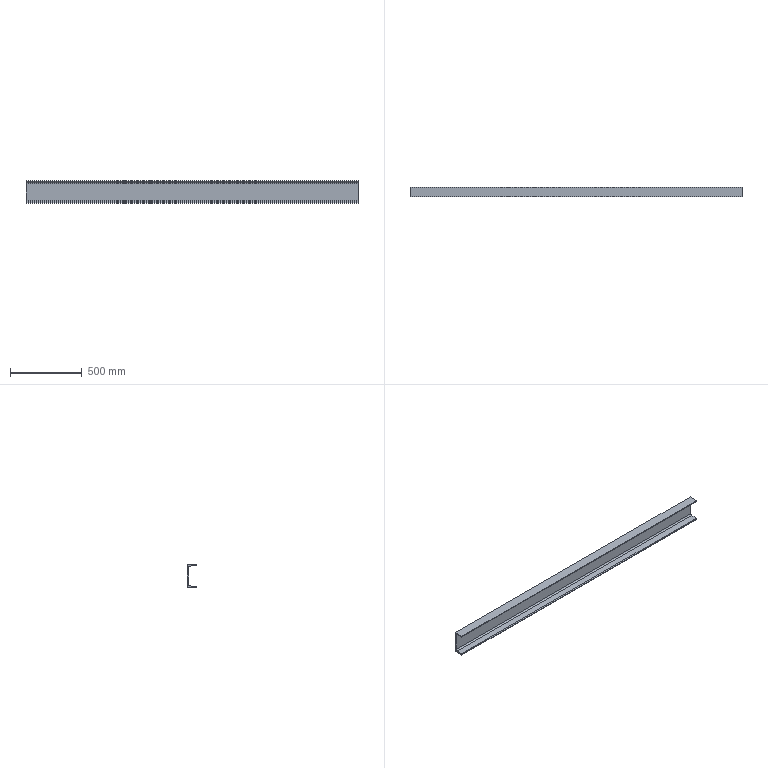Part | STEP file | 08-Channel 100x48_default<machining> | 1 solid | 14 faces | box 2320 x 65 x 160 mm | volume 5777947 mm3 | plane 10 | cylinder 4 | commonest cylinder face diameters 10 x2 20 x2
STEP:
#1=CARTESIAN_POINT('',(0.,0.,0.));
#2=DIRECTION('',(0.,0.,1.));
#3=DIRECTION('',(1.,0.,0.));
#4=AXIS2_PLACEMENT_3D('',#1,#2,#3);
#5=CARTESIAN_POINT('',(0.,-65.,-160.));
#6=VERTEX_POINT('',#5);
#7=CARTESIAN_POINT('',(0.,0.,-160.));
#8=VERTEX_POINT('',#7);
#9=CARTESIAN_POINT('',(0.,0.,-160.));
#10=DIRECTION('',(0.,1.,0.));
#11=VECTOR('',#10,1.);
#12=LINE('',#9,#11);
#13=CARTESIAN_POINT('',(2320.,0.,-160.));
#14=DIRECTION('',(0.,0.,1.));
#15=DIRECTION('',(1.,0.,0.));
#16=AXIS2_PLACEMENT_3D('',#13,#14,#15);
#17=PLANE('',#16);
#18=CARTESIAN_POINT('',(-2320.,0.));
#19=DIRECTION('',(0.,1.));
#20=VECTOR('',#19,1.);
#21=LINE('',#18,#20);
#22=(GEOMETRIC_REPRESENTATION_CONTEXT(2)PARAMETRIC_REPRESENTATION_CONTEXT()REPRESENTATION_CONTEXT('',''));
#23=DEFINITIONAL_REPRESENTATION('',(#21),#22);
#24=PCURVE('',#17,#23);
#25=CARTESIAN_POINT('',(0.,-60.,-156.59));
#26=DIRECTION('',(1.,0.,0.));
#27=DIRECTION('',(0.,0.,-1.));
#28=AXIS2_PLACEMENT_3D('',#25,#26,#27);
#29=PLANE('',#28);
#30=CARTESIAN_POINT('',(3.41,60.));
#31=DIRECTION('',(0.,1.));
#32=VECTOR('',#31,1.);
#33=LINE('',#30,#32);
#34=(GEOMETRIC_REPRESENTATION_CONTEXT(2)PARAMETRIC_REPRESENTATION_CONTEXT()REPRESENTATION_CONTEXT('',''));
#35=DEFINITIONAL_REPRESENTATION('',(#33),#34);
#36=PCURVE('',#29,#35);
#37=SURFACE_CURVE('',#12,(#24,#36),.PCURVE_S1.);
#38=EDGE_CURVE('',#6,#8,#37,.T.);
#39=ORIENTED_EDGE('',*,*,#38,.T.);
#40=CARTESIAN_POINT('',(2320.,0.,-160.));
#41=VERTEX_POINT('',#40);
#42=CARTESIAN_POINT('',(2320.,0.,-160.));
#43=DIRECTION('',(-1.,0.,0.));
#44=VECTOR('',#43,1.);
#45=LINE('',#42,#44);
#46=CARTESIAN_POINT('',(0.,0.));
#47=DIRECTION('',(-1.,0.));
#48=VECTOR('',#47,1.);
#49=LINE('',#46,#48);
#50=(GEOMETRIC_REPRESENTATION_CONTEXT(2)PARAMETRIC_REPRESENTATION_CONTEXT()REPRESENTATION_CONTEXT('',''));
#51=DEFINITIONAL_REPRESENTATION('',(#49),#50);
#52=PCURVE('',#17,#51);
#53=CARTESIAN_POINT('',(2320.,0.,0.));
#54=DIRECTION('',(0.,-1.,0.));
#55=DIRECTION('',(0.,0.,-1.));
#56=AXIS2_PLACEMENT_3D('',#53,#54,#55);
#57=PLANE('',#56);
#58=CARTESIAN_POINT('',(160.,0.));
#59=DIRECTION('',(0.,-1.));
#60=VECTOR('',#59,1.);
#61=LINE('',#58,#60);
#62=(GEOMETRIC_REPRESENTATION_CONTEXT(2)PARAMETRIC_REPRESENTATION_CONTEXT()REPRESENTATION_CONTEXT('',''));
#63=DEFINITIONAL_REPRESENTATION('',(#61),#62);
#64=PCURVE('',#57,#63);
#65=SURFACE_CURVE('',#45,(#52,#64),.PCURVE_S1.);
#66=EDGE_CURVE('',#41,#8,#65,.T.);
#67=ORIENTED_EDGE('',*,*,#66,.F.);
#68=CARTESIAN_POINT('',(2320.,-65.,-160.));
#69=VERTEX_POINT('',#68);
#70=CARTESIAN_POINT('',(2320.,0.,-160.));
#71=DIRECTION('',(0.,1.,0.));
#72=VECTOR('',#71,1.);
#73=LINE('',#70,#72);
#74=CARTESIAN_POINT('',(0.,0.));
#75=DIRECTION('',(0.,1.));
#76=VECTOR('',#75,1.);
#77=LINE('',#74,#76);
#78=(GEOMETRIC_REPRESENTATION_CONTEXT(2)PARAMETRIC_REPRESENTATION_CONTEXT()REPRESENTATION_CONTEXT('',''));
#79=DEFINITIONAL_REPRESENTATION('',(#77),#78);
#80=PCURVE('',#17,#79);
#81=CARTESIAN_POINT('',(2320.,-60.,-156.59));
#82=DIRECTION('',(1.,0.,0.));
#83=DIRECTION('',(0.,0.,-1.));
#84=AXIS2_PLACEMENT_3D('',#81,#82,#83);
#85=PLANE('',#84);
#86=CARTESIAN_POINT('',(3.41,60.));
#87=DIRECTION('',(0.,1.));
#88=VECTOR('',#87,1.);
#89=LINE('',#86,#88);
#90=(GEOMETRIC_REPRESENTATION_CONTEXT(2)PARAMETRIC_REPRESENTATION_CONTEXT()REPRESENTATION_CONTEXT('',''));
#91=DEFINITIONAL_REPRESENTATION('',(#89),#90);
#92=PCURVE('',#85,#91);
#93=SURFACE_CURVE('',#73,(#80,#92),.PCURVE_S1.);
#94=EDGE_CURVE('',#69,#41,#93,.T.);
#95=ORIENTED_EDGE('',*,*,#94,.F.);
#96=CARTESIAN_POINT('',(2320.,-65.,-160.));
#97=DIRECTION('',(-1.,0.,0.));
#98=VECTOR('',#97,1.);
#99=LINE('',#96,#98);
#100=CARTESIAN_POINT('',(0.,-65.));
#101=DIRECTION('',(-1.,0.));
#102=VECTOR('',#101,1.);
#103=LINE('',#100,#102);
#104=(GEOMETRIC_REPRESENTATION_CONTEXT(2)PARAMETRIC_REPRESENTATION_CONTEXT()REPRESENTATION_CONTEXT('',''));
#105=DEFINITIONAL_REPRESENTATION('',(#103),#104);
#106=PCURVE('',#17,#105);
#107=CARTESIAN_POINT('',(2320.,-65.,-156.59));
#108=DIRECTION('',(0.,1.,0.));
#109=DIRECTION('',(0.,0.,1.));
#110=AXIS2_PLACEMENT_3D('',#107,#108,#109);
#111=PLANE('',#110);
#112=CARTESIAN_POINT('',(-3.41,0.));
#113=DIRECTION('',(0.,-1.));
#114=VECTOR('',#113,1.);
#115=LINE('',#112,#114);
#116=(GEOMETRIC_REPRESENTATION_CONTEXT(2)PARAMETRIC_REPRESENTATION_CONTEXT()REPRESENTATION_CONTEXT('',''));
#117=DEFINITIONAL_REPRESENTATION('',(#115),#116);
#118=PCURVE('',#111,#117);
#119=SURFACE_CURVE('',#99,(#106,#118),.PCURVE_S1.);
#120=EDGE_CURVE('',#69,#6,#119,.T.);
#121=ORIENTED_EDGE('',*,*,#120,.T.);
#122=EDGE_LOOP('',(#39,#67,#95,#121));
#123=FACE_BOUND('',#122,.T.);
#124=ADVANCED_FACE('',(#123),#17,.F.);
#125=CARTESIAN_POINT('',(0.,0.,0.));
#126=VERTEX_POINT('',#125);
#127=CARTESIAN_POINT('',(0.,0.,0.));
#128=DIRECTION('',(0.,0.,1.));
#129=VECTOR('',#128,1.);
#130=LINE('',#127,#129);
#131=CARTESIAN_POINT('',(0.,-2320.));
#132=DIRECTION('',(-1.,0.));
#133=VECTOR('',#132,1.);
#134=LINE('',#131,#133);
#135=(GEOMETRIC_REPRESENTATION_CONTEXT(2)PARAMETRIC_REPRESENTATION_CONTEXT()REPRESENTATION_CONTEXT('',''));
#136=DEFINITIONAL_REPRESENTATION('',(#134),#135);
#137=PCURVE('',#57,#136);
#138=CARTESIAN_POINT('',(-156.59,60.));
#139=DIRECTION('',(-1.,0.));
#140=VECTOR('',#139,1.);
#141=LINE('',#138,#140);
#142=(GEOMETRIC_REPRESENTATION_CONTEXT(2)PARAMETRIC_REPRESENTATION_CONTEXT()REPRESENTATION_CONTEXT('',''));
#143=DEFINITIONAL_REPRESENTATION('',(#141),#142);
#144=PCURVE('',#29,#143);
#145=SURFACE_CURVE('',#130,(#137,#144),.PCURVE_S1.);
#146=EDGE_CURVE('',#8,#126,#145,.T.);
#147=ORIENTED_EDGE('',*,*,#146,.T.);
#148=CARTESIAN_POINT('',(2320.,0.,0.));
#149=VERTEX_POINT('',#148);
#150=CARTESIAN_POINT('',(2320.,0.,0.));
#151=DIRECTION('',(-1.,0.,0.));
#152=VECTOR('',#151,1.);
#153=LINE('',#150,#152);
#154=CARTESIAN_POINT('',(0.,0.));
#155=DIRECTION('',(0.,-1.));
#156=VECTOR('',#155,1.);
#157=LINE('',#154,#156);
#158=(GEOMETRIC_REPRESENTATION_CONTEXT(2)PARAMETRIC_REPRESENTATION_CONTEXT()REPRESENTATION_CONTEXT('',''));
#159=DEFINITIONAL_REPRESENTATION('',(#157),#158);
#160=PCURVE('',#57,#159);
#161=CARTESIAN_POINT('',(2320.,0.,0.));
#162=DIRECTION('',(0.,0.,-1.));
#163=DIRECTION('',(0.,1.,0.));
#164=AXIS2_PLACEMENT_3D('',#161,#162,#163);
#165=PLANE('',#164);
#166=CARTESIAN_POINT('',(0.,0.));
#167=DIRECTION('',(0.,-1.));
#168=VECTOR('',#167,1.);
#169=LINE('',#166,#168);
#170=(GEOMETRIC_REPRESENTATION_CONTEXT(2)PARAMETRIC_REPRESENTATION_CONTEXT()REPRESENTATION_CONTEXT('',''));
#171=DEFINITIONAL_REPRESENTATION('',(#169),#170);
#172=PCURVE('',#165,#171);
#173=SURFACE_CURVE('',#153,(#160,#172),.PCURVE_S1.);
#174=EDGE_CURVE('',#149,#126,#173,.T.);
#175=ORIENTED_EDGE('',*,*,#174,.F.);
#176=CARTESIAN_POINT('',(2320.,0.,0.));
#177=DIRECTION('',(0.,0.,1.));
#178=VECTOR('',#177,1.);
#179=LINE('',#176,#178);
#180=CARTESIAN_POINT('',(0.,0.));
#181=DIRECTION('',(-1.,0.));
#182=VECTOR('',#181,1.);
#183=LINE('',#180,#182);
#184=(GEOMETRIC_REPRESENTATION_CONTEXT(2)PARAMETRIC_REPRESENTATION_CONTEXT()REPRESENTATION_CONTEXT('',''));
#185=DEFINITIONAL_REPRESENTATION('',(#183),#184);
#186=PCURVE('',#57,#185);
#187=CARTESIAN_POINT('',(-156.59,60.));
#188=DIRECTION('',(-1.,0.));
#189=VECTOR('',#188,1.);
#190=LINE('',#187,#189);
#191=(GEOMETRIC_REPRESENTATION_CONTEXT(2)PARAMETRIC_REPRESENTATION_CONTEXT()REPRESENTATION_CONTEXT('',''));
#192=DEFINITIONAL_REPRESENTATION('',(#190),#191);
#193=PCURVE('',#85,#192);
#194=SURFACE_CURVE('',#179,(#186,#193),.PCURVE_S1.);
#195=EDGE_CURVE('',#41,#149,#194,.T.);
#196=ORIENTED_EDGE('',*,*,#195,.F.);
#197=ORIENTED_EDGE('',*,*,#66,.T.);
#198=EDGE_LOOP('',(#147,#175,#196,#197));
#199=FACE_BOUND('',#198,.T.);
#200=ADVANCED_FACE('',(#199),#57,.F.);
#201=CARTESIAN_POINT('',(0.,-65.,0.));
#202=VERTEX_POINT('',#201);
#203=CARTESIAN_POINT('',(0.,0.,0.));
#204=DIRECTION('',(0.,-1.,0.));
#205=VECTOR('',#204,1.);
#206=LINE('',#203,#205);
#207=CARTESIAN_POINT('',(0.,-2320.));
#208=DIRECTION('',(-1.,0.));
#209=VECTOR('',#208,1.);
#210=LINE('',#207,#209);
#211=(GEOMETRIC_REPRESENTATION_CONTEXT(2)PARAMETRIC_REPRESENTATION_CONTEXT()REPRESENTATION_CONTEXT('',''));
#212=DEFINITIONAL_REPRESENTATION('',(#210),#211);
#213=PCURVE('',#165,#212);
#214=CARTESIAN_POINT('',(-156.59,60.));
#215=DIRECTION('',(0.,-1.));
#216=VECTOR('',#215,1.);
#217=LINE('',#214,#216);
#218=(GEOMETRIC_REPRESENTATION_CONTEXT(2)PARAMETRIC_REPRESENTATION_CONTEXT()REPRESENTATION_CONTEXT('',''));
#219=DEFINITIONAL_REPRESENTATION('',(#217),#218);
#220=PCURVE('',#29,#219);
#221=SURFACE_CURVE('',#206,(#213,#220),.PCURVE_S1.);
#222=EDGE_CURVE('',#126,#202,#221,.T.);
#223=ORIENTED_EDGE('',*,*,#222,.T.);
#224=CARTESIAN_POINT('',(2320.,-65.,0.));
#225=VERTEX_POINT('',#224);
#226=CARTESIAN_POINT('',(2320.,-65.,0.));
#227=DIRECTION('',(-1.,0.,0.));
#228=VECTOR('',#227,1.);
#229=LINE('',#226,#228);
#230=CARTESIAN_POINT('',(-65.,0.));
#231=DIRECTION('',(0.,-1.));
#232=VECTOR('',#231,1.);
#233=LINE('',#230,#232);
#234=(GEOMETRIC_REPRESENTATION_CONTEXT(2)PARAMETRIC_REPRESENTATION_CONTEXT()REPRESENTATION_CONTEXT('',''));
#235=DEFINITIONAL_REPRESENTATION('',(#233),#234);
#236=PCURVE('',#165,#235);
#237=CARTESIAN_POINT('',(2320.,-65.,-3.41));
#238=DIRECTION('',(0.,1.,0.));
#239=DIRECTION('',(0.,0.,1.));
#240=AXIS2_PLACEMENT_3D('',#237,#238,#239);
#241=PLANE('',#240);
#242=CARTESIAN_POINT('',(3.41,0.));
#243=DIRECTION('',(0.,-1.));
#244=VECTOR('',#243,1.);
#245=LINE('',#242,#244);
#246=(GEOMETRIC_REPRESENTATION_CONTEXT(2)PARAMETRIC_REPRESENTATION_CONTEXT()REPRESENTATION_CONTEXT('',''));
#247=DEFINITIONAL_REPRESENTATION('',(#245),#246);
#248=PCURVE('',#241,#247);
#249=SURFACE_CURVE('',#229,(#236,#248),.PCURVE_S1.);
#250=EDGE_CURVE('',#225,#202,#249,.T.);
#251=ORIENTED_EDGE('',*,*,#250,.F.);
#252=CARTESIAN_POINT('',(2320.,0.,0.));
#253=DIRECTION('',(0.,-1.,0.));
#254=VECTOR('',#253,1.);
#255=LINE('',#252,#254);
#256=CARTESIAN_POINT('',(0.,0.));
#257=DIRECTION('',(-1.,0.));
#258=VECTOR('',#257,1.);
#259=LINE('',#256,#258);
#260=(GEOMETRIC_REPRESENTATION_CONTEXT(2)PARAMETRIC_REPRESENTATION_CONTEXT()REPRESENTATION_CONTEXT('',''));
#261=DEFINITIONAL_REPRESENTATION('',(#259),#260);
#262=PCURVE('',#165,#261);
#263=CARTESIAN_POINT('',(-156.59,60.));
#264=DIRECTION('',(0.,-1.));
#265=VECTOR('',#264,1.);
#266=LINE('',#263,#265);
#267=(GEOMETRIC_REPRESENTATION_CONTEXT(2)PARAMETRIC_REPRESENTATION_CONTEXT()REPRESENTATION_CONTEXT('',''));
#268=DEFINITIONAL_REPRESENTATION('',(#266),#267);
#269=PCURVE('',#85,#268);
#270=SURFACE_CURVE('',#255,(#262,#269),.PCURVE_S1.);
#271=EDGE_CURVE('',#149,#225,#270,.T.);
#272=ORIENTED_EDGE('',*,*,#271,.F.);
#273=ORIENTED_EDGE('',*,*,#174,.T.);
#274=EDGE_LOOP('',(#223,#251,#272,#273));
#275=FACE_BOUND('',#274,.T.);
#276=ADVANCED_FACE('',(#275),#165,.F.);
#277=CARTESIAN_POINT('',(0.,-65.,-3.41));
#278=VERTEX_POINT('',#277);
#279=CARTESIAN_POINT('',(0.,-65.,-3.41));
#280=DIRECTION('',(0.,0.,-1.));
#281=VECTOR('',#280,1.);
#282=LINE('',#279,#281);
#283=CARTESIAN_POINT('',(0.,-2320.));
#284=DIRECTION('',(-1.,0.));
#285=VECTOR('',#284,1.);
#286=LINE('',#283,#285);
#287=(GEOMETRIC_REPRESENTATION_CONTEXT(2)PARAMETRIC_REPRESENTATION_CONTEXT()REPRESENTATION_CONTEXT('',''));
#288=DEFINITIONAL_REPRESENTATION('',(#286),#287);
#289=PCURVE('',#241,#288);
#290=CARTESIAN_POINT('',(-153.18,-5.));
#291=DIRECTION('',(1.,0.));
#292=VECTOR('',#291,1.);
#293=LINE('',#290,#292);
#294=(GEOMETRIC_REPRESENTATION_CONTEXT(2)PARAMETRIC_REPRESENTATION_CONTEXT()REPRESENTATION_CONTEXT('',''));
#295=DEFINITIONAL_REPRESENTATION('',(#293),#294);
#296=PCURVE('',#29,#295);
#297=SURFACE_CURVE('',#282,(#289,#296),.PCURVE_S1.);
#298=EDGE_CURVE('',#202,#278,#297,.T.);
#299=ORIENTED_EDGE('',*,*,#298,.T.);
#300=CARTESIAN_POINT('',(2320.,-65.,-3.41));
#301=VERTEX_POINT('',#300);
#302=CARTESIAN_POINT('',(2320.,-65.,-3.41));
#303=DIRECTION('',(-1.,0.,0.));
#304=VECTOR('',#303,1.);
#305=LINE('',#302,#304);
#306=CARTESIAN_POINT('',(0.,0.));
#307=DIRECTION('',(0.,-1.));
#308=VECTOR('',#307,1.);
#309=LINE('',#306,#308);
#310=(GEOMETRIC_REPRESENTATION_CONTEXT(2)PARAMETRIC_REPRESENTATION_CONTEXT()REPRESENTATION_CONTEXT('',''));
#311=DEFINITIONAL_REPRESENTATION('',(#309),#310);
#312=PCURVE('',#241,#311);
#313=CARTESIAN_POINT('',(2320.,-60.,-3.41));
#314=DIRECTION('',(-1.,0.,0.));
#315=DIRECTION('',(0.,0.,1.));
#316=AXIS2_PLACEMENT_3D('',#313,#314,#315);
#317=CYLINDRICAL_SURFACE('',#316,5.);
#318=CARTESIAN_POINT('',(4.712,0.));
#319=DIRECTION('',(0.,1.));
#320=VECTOR('',#319,1.);
#321=LINE('',#318,#320);
#322=(GEOMETRIC_REPRESENTATION_CONTEXT(2)PARAMETRIC_REPRESENTATION_CONTEXT()REPRESENTATION_CONTEXT('',''));
#323=DEFINITIONAL_REPRESENTATION('',(#321),#322);
#324=PCURVE('',#317,#323);
#325=SURFACE_CURVE('',#305,(#312,#324),.PCURVE_S1.);
#326=EDGE_CURVE('',#301,#278,#325,.T.);
#327=ORIENTED_EDGE('',*,*,#326,.F.);
#328=CARTESIAN_POINT('',(2320.,-65.,-3.41));
#329=DIRECTION('',(0.,0.,-1.));
#330=VECTOR('',#329,1.);
#331=LINE('',#328,#330);
#332=CARTESIAN_POINT('',(0.,0.));
#333=DIRECTION('',(-1.,0.));
#334=VECTOR('',#333,1.);
#335=LINE('',#332,#334);
#336=(GEOMETRIC_REPRESENTATION_CONTEXT(2)PARAMETRIC_REPRESENTATION_CONTEXT()REPRESENTATION_CONTEXT('',''));
#337=DEFINITIONAL_REPRESENTATION('',(#335),#336);
#338=PCURVE('',#241,#337);
#339=CARTESIAN_POINT('',(-153.18,-5.));
#340=DIRECTION('',(1.,0.));
#341=VECTOR('',#340,1.);
#342=LINE('',#339,#341);
#343=(GEOMETRIC_REPRESENTATION_CONTEXT(2)PARAMETRIC_REPRESENTATION_CONTEXT()REPRESENTATION_CONTEXT('',''));
#344=DEFINITIONAL_REPRESENTATION('',(#342),#343);
#345=PCURVE('',#85,#344);
#346=SURFACE_CURVE('',#331,(#338,#345),.PCURVE_S1.);
#347=EDGE_CURVE('',#225,#301,#346,.T.);
#348=ORIENTED_EDGE('',*,*,#347,.F.);
#349=ORIENTED_EDGE('',*,*,#250,.T.);
#350=EDGE_LOOP('',(#299,#327,#348,#349));
#351=FACE_BOUND('',#350,.T.);
#352=ADVANCED_FACE('',(#351),#241,.F.);
#353=CARTESIAN_POINT('',(0.,-60.287,-8.402));
#354=VERTEX_POINT('',#353);
#355=CARTESIAN_POINT('',(0.,-60.,-3.41));
#356=DIRECTION('',(1.,0.,0.));
#357=DIRECTION('',(0.,0.,-1.));
#358=AXIS2_PLACEMENT_3D('',#355,#356,#357);
#359=CIRCLE('',#358,5.);
#360=CARTESIAN_POINT('',(9.425,2320.));
#361=DIRECTION('',(-1.,0.));
#362=VECTOR('',#361,1.);
#363=LINE('',#360,#362);
#364=(GEOMETRIC_REPRESENTATION_CONTEXT(2)PARAMETRIC_REPRESENTATION_CONTEXT()REPRESENTATION_CONTEXT('',''));
#365=DEFINITIONAL_REPRESENTATION('',(#363),#364);
#366=PCURVE('',#317,#365);
#367=CARTESIAN_POINT('',(-153.18,0.));
#368=DIRECTION('',(1.,0.));
#369=AXIS2_PLACEMENT_2D('',#367,#368);
#370=CIRCLE('',#369,5.);
#371=(GEOMETRIC_REPRESENTATION_CONTEXT(2)PARAMETRIC_REPRESENTATION_CONTEXT()REPRESENTATION_CONTEXT('',''));
#372=DEFINITIONAL_REPRESENTATION('',(#370),#371);
#373=PCURVE('',#29,#372);
#374=SURFACE_CURVE('',#359,(#366,#373),.PCURVE_S1.);
#375=EDGE_CURVE('',#278,#354,#374,.T.);
#376=ORIENTED_EDGE('',*,*,#375,.T.);
#377=CARTESIAN_POINT('',(2320.,-60.287,-8.402));
#378=VERTEX_POINT('',#377);
#379=CARTESIAN_POINT('',(2320.,-60.287,-8.402));
#380=DIRECTION('',(-1.,0.,0.));
#381=VECTOR('',#380,1.);
#382=LINE('',#379,#381);
#383=CARTESIAN_POINT('',(3.199,0.));
#384=DIRECTION('',(0.,1.));
#385=VECTOR('',#384,1.);
#386=LINE('',#383,#385);
#387=(GEOMETRIC_REPRESENTATION_CONTEXT(2)PARAMETRIC_REPRESENTATION_CONTEXT()REPRESENTATION_CONTEXT('',''));
#388=DEFINITIONAL_REPRESENTATION('',(#386),#387);
#389=PCURVE('',#317,#388);
#390=CARTESIAN_POINT('',(2320.,-17.926,-10.838));
#391=DIRECTION('',(0.,0.05743,0.9983));
#392=DIRECTION('',(0.,-0.9983,0.05743));
#393=AXIS2_PLACEMENT_3D('',#390,#391,#392);
#394=PLANE('',#393);
#395=CARTESIAN_POINT('',(42.431,0.));
#396=DIRECTION('',(0.,-1.));
#397=VECTOR('',#396,1.);
#398=LINE('',#395,#397);
#399=(GEOMETRIC_REPRESENTATION_CONTEXT(2)PARAMETRIC_REPRESENTATION_CONTEXT()REPRESENTATION_CONTEXT('',''));
#400=DEFINITIONAL_REPRESENTATION('',(#398),#399);
#401=PCURVE('',#394,#400);
#402=SURFACE_CURVE('',#382,(#389,#401),.PCURVE_S1.);
#403=EDGE_CURVE('',#378,#354,#402,.T.);
#404=ORIENTED_EDGE('',*,*,#403,.F.);
#405=CARTESIAN_POINT('',(2320.,-60.,-3.41));
#406=DIRECTION('',(1.,0.,0.));
#407=DIRECTION('',(0.,0.,-1.));
#408=AXIS2_PLACEMENT_3D('',#405,#406,#407);
#409=CIRCLE('',#408,5.);
#410=CARTESIAN_POINT('',(9.425,0.));
#411=DIRECTION('',(-1.,0.));
#412=VECTOR('',#411,1.);
#413=LINE('',#410,#412);
#414=(GEOMETRIC_REPRESENTATION_CONTEXT(2)PARAMETRIC_REPRESENTATION_CONTEXT()REPRESENTATION_CONTEXT('',''));
#415=DEFINITIONAL_REPRESENTATION('',(#413),#414);
#416=PCURVE('',#317,#415);
#417=CARTESIAN_POINT('',(-153.18,0.));
#418=DIRECTION('',(1.,0.));
#419=AXIS2_PLACEMENT_2D('',#417,#418);
#420=CIRCLE('',#419,5.);
#421=(GEOMETRIC_REPRESENTATION_CONTEXT(2)PARAMETRIC_REPRESENTATION_CONTEXT()REPRESENTATION_CONTEXT('',''));
#422=DEFINITIONAL_REPRESENTATION('',(#420),#421);
#423=PCURVE('',#85,#422);
#424=SURFACE_CURVE('',#409,(#416,#423),.PCURVE_S1.);
#425=EDGE_CURVE('',#301,#378,#424,.T.);
#426=ORIENTED_EDGE('',*,*,#425,.F.);
#427=ORIENTED_EDGE('',*,*,#326,.T.);
#428=EDGE_LOOP('',(#376,#404,#426,#427));
#429=FACE_BOUND('',#428,.T.);
#430=ADVANCED_FACE('',(#429),#317,.T.);
#431=CARTESIAN_POINT('',(0.,-17.926,-10.838));
#432=VERTEX_POINT('',#431);
#433=CARTESIAN_POINT('',(0.,-17.926,-10.838));
#434=DIRECTION('',(0.,0.9983,-0.05743));
#435=VECTOR('',#434,1.);
#436=LINE('',#433,#435);
#437=CARTESIAN_POINT('',(0.,-2320.));
#438=DIRECTION('',(-1.,0.));
#439=VECTOR('',#438,1.);
#440=LINE('',#437,#439);
#441=(GEOMETRIC_REPRESENTATION_CONTEXT(2)PARAMETRIC_REPRESENTATION_CONTEXT()REPRESENTATION_CONTEXT('',''));
#442=DEFINITIONAL_REPRESENTATION('',(#440),#441);
#443=PCURVE('',#394,#442);
#444=CARTESIAN_POINT('',(-145.752,42.074));
#445=DIRECTION('',(0.05743,0.9983));
#446=VECTOR('',#445,1.);
#447=LINE('',#444,#446);
#448=(GEOMETRIC_REPRESENTATION_CONTEXT(2)PARAMETRIC_REPRESENTATION_CONTEXT()REPRESENTATION_CONTEXT('',''));
#449=DEFINITIONAL_REPRESENTATION('',(#447),#448);
#450=PCURVE('',#29,#449);
#451=SURFACE_CURVE('',#436,(#443,#450),.PCURVE_S1.);
#452=EDGE_CURVE('',#354,#432,#451,.T.);
#453=ORIENTED_EDGE('',*,*,#452,.T.);
#454=CARTESIAN_POINT('',(2320.,-17.926,-10.838));
#455=VERTEX_POINT('',#454);
#456=CARTESIAN_POINT('',(2320.,-17.926,-10.838));
#457=DIRECTION('',(-1.,0.,0.));
#458=VECTOR('',#457,1.);
#459=LINE('',#456,#458);
#460=CARTESIAN_POINT('',(0.,0.));
#461=DIRECTION('',(0.,-1.));
#462=VECTOR('',#461,1.);
#463=LINE('',#460,#462);
#464=(GEOMETRIC_REPRESENTATION_CONTEXT(2)PARAMETRIC_REPRESENTATION_CONTEXT()REPRESENTATION_CONTEXT('',''));
#465=DEFINITIONAL_REPRESENTATION('',(#463),#464);
#466=PCURVE('',#394,#465);
#467=CARTESIAN_POINT('',(2320.,-18.5,-20.822));
#468=DIRECTION('',(-1.,0.,0.));
#469=DIRECTION('',(0.,0.,1.));
#470=AXIS2_PLACEMENT_3D('',#467,#468,#469);
#471=CYLINDRICAL_SURFACE('',#470,10.);
#472=CARTESIAN_POINT('',(0.05746,0.));
#473=DIRECTION('',(0.,1.));
#474=VECTOR('',#473,1.);
#475=LINE('',#472,#474);
#476=(GEOMETRIC_REPRESENTATION_CONTEXT(2)PARAMETRIC_REPRESENTATION_CONTEXT()REPRESENTATION_CONTEXT('',''));
#477=DEFINITIONAL_REPRESENTATION('',(#475),#476);
#478=PCURVE('',#471,#477);
#479=SURFACE_CURVE('',#459,(#466,#478),.PCURVE_S1.);
#480=EDGE_CURVE('',#455,#432,#479,.T.);
#481=ORIENTED_EDGE('',*,*,#480,.F.);
#482=CARTESIAN_POINT('',(2320.,-17.926,-10.838));
#483=DIRECTION('',(0.,0.9983,-0.05743));
#484=VECTOR('',#483,1.);
#485=LINE('',#482,#484);
#486=CARTESIAN_POINT('',(0.,0.));
#487=DIRECTION('',(-1.,0.));
#488=VECTOR('',#487,1.);
#489=LINE('',#486,#488);
#490=(GEOMETRIC_REPRESENTATION_CONTEXT(2)PARAMETRIC_REPRESENTATION_CONTEXT()REPRESENTATION_CONTEXT('',''));
#491=DEFINITIONAL_REPRESENTATION('',(#489),#490);
#492=PCURVE('',#394,#491);
#493=CARTESIAN_POINT('',(-145.752,42.074));
#494=DIRECTION('',(0.05743,0.9983));
#495=VECTOR('',#494,1.);
#496=LINE('',#493,#495);
#497=(GEOMETRIC_REPRESENTATION_CONTEXT(2)PARAMETRIC_REPRESENTATION_CONTEXT()REPRESENTATION_CONTEXT('',''));
#498=DEFINITIONAL_REPRESENTATION('',(#496),#497);
#499=PCURVE('',#85,#498);
#500=SURFACE_CURVE('',#485,(#492,#499),.PCURVE_S1.);
#501=EDGE_CURVE('',#378,#455,#500,.T.);
#502=ORIENTED_EDGE('',*,*,#501,.F.);
#503=ORIENTED_EDGE('',*,*,#403,.T.);
#504=EDGE_LOOP('',(#453,#481,#502,#503));
#505=FACE_BOUND('',#504,.T.);
#506=ADVANCED_FACE('',(#505),#394,.F.);
#507=ORIENTED_EDGE('',*,*,#480,.F.);
#508=CARTESIAN_POINT('',(2320.,-8.5,-20.822));
#509=VERTEX_POINT('',#508);
#510=CARTESIAN_POINT('',(2320.,-18.5,-20.822));
#511=DIRECTION('',(-1.,0.,0.));
#512=DIRECTION('',(0.,0.,1.));
#513=AXIS2_PLACEMENT_3D('',#510,#511,#512);
#514=CIRCLE('',#513,10.);
#515=CARTESIAN_POINT('',(0.,0.));
#516=DIRECTION('',(1.,0.));
#517=VECTOR('',#516,1.);
#518=LINE('',#515,#517);
#519=(GEOMETRIC_REPRESENTATION_CONTEXT(2)PARAMETRIC_REPRESENTATION_CONTEXT()REPRESENTATION_CONTEXT('',''));
#520=DEFINITIONAL_REPRESENTATION('',(#518),#519);
#521=PCURVE('',#471,#520);
#522=CARTESIAN_POINT('',(-145.768,41.5));
#523=CARTESIAN_POINT('',(-145.768,58.821));
#524=CARTESIAN_POINT('',(-130.768,50.16));
#525=CARTESIAN_POINT('',(-115.768,41.5));
#526=CARTESIAN_POINT('',(-130.768,32.84));
#527=CARTESIAN_POINT('',(-145.768,24.179));
#528=CARTESIAN_POINT('',(-145.768,41.5));
#529=(BOUNDED_CURVE()B_SPLINE_CURVE(2,(#522,#523,#524,#525,#526,#527,#528),.UNSPECIFIED.,.T.,.F.)B_SPLINE_CURVE_WITH_KNOTS((1,2,2,2,2,1),(-2.094,0.,2.094,4.189,6.283,8.378),.UNSPECIFIED.)CURVE()GEOMETRIC_REPRESENTATION_ITEM()RATIONAL_B_SPLINE_CURVE((1.,0.5,1.,0.5,1.,0.5,1.))REPRESENTATION_ITEM(''));
#530=(GEOMETRIC_REPRESENTATION_CONTEXT(2)PARAMETRIC_REPRESENTATION_CONTEXT()REPRESENTATION_CONTEXT('',''));
#531=DEFINITIONAL_REPRESENTATION('',(#529),#530);
#532=PCURVE('',#85,#531);
#533=SURFACE_CURVE('',#514,(#521,#532),.PCURVE_S1.);
#534=EDGE_CURVE('',#455,#509,#533,.T.);
#535=ORIENTED_EDGE('',*,*,#534,.T.);
#536=CARTESIAN_POINT('',(0.,-8.5,-20.822));
#537=VERTEX_POINT('',#536);
#538=CARTESIAN_POINT('',(2320.,-8.5,-20.822));
#539=DIRECTION('',(-1.,0.,0.));
#540=VECTOR('',#539,1.);
#541=LINE('',#538,#540);
#542=CARTESIAN_POINT('',(1.571,0.));
#543=DIRECTION('',(0.,1.));
#544=VECTOR('',#543,1.);
#545=LINE('',#542,#544);
#546=(GEOMETRIC_REPRESENTATION_CONTEXT(2)PARAMETRIC_REPRESENTATION_CONTEXT()REPRESENTATION_CONTEXT('',''));
#547=DEFINITIONAL_REPRESENTATION('',(#545),#546);
#548=PCURVE('',#471,#547);
#549=CARTESIAN_POINT('',(2320.,-8.5,-139.178));
#550=DIRECTION('',(0.,1.,0.));
#551=DIRECTION('',(0.,0.,1.));
#552=AXIS2_PLACEMENT_3D('',#549,#550,#551);
#553=PLANE('',#552);
#554=CARTESIAN_POINT('',(118.356,0.));
#555=DIRECTION('',(0.,-1.));
#556=VECTOR('',#555,1.);
#557=LINE('',#554,#556);
#558=(GEOMETRIC_REPRESENTATION_CONTEXT(2)PARAMETRIC_REPRESENTATION_CONTEXT()REPRESENTATION_CONTEXT('',''));
#559=DEFINITIONAL_REPRESENTATION('',(#557),#558);
#560=PCURVE('',#553,#559);
#561=SURFACE_CURVE('',#541,(#548,#560),.PCURVE_S1.);
#562=EDGE_CURVE('',#509,#537,#561,.T.);
#563=ORIENTED_EDGE('',*,*,#562,.T.);
#564=CARTESIAN_POINT('',(0.,-18.5,-20.822));
#565=DIRECTION('',(-1.,0.,0.));
#566=DIRECTION('',(0.,0.,1.));
#567=AXIS2_PLACEMENT_3D('',#564,#565,#566);
#568=CIRCLE('',#567,10.);
#569=CARTESIAN_POINT('',(0.,2320.));
#570=DIRECTION('',(1.,0.));
#571=VECTOR('',#570,1.);
#572=LINE('',#569,#571);
#573=(GEOMETRIC_REPRESENTATION_CONTEXT(2)PARAMETRIC_REPRESENTATION_CONTEXT()REPRESENTATION_CONTEXT('',''));
#574=DEFINITIONAL_REPRESENTATION('',(#572),#573);
#575=PCURVE('',#471,#574);
#576=CARTESIAN_POINT('',(-145.768,41.5));
#577=CARTESIAN_POINT('',(-145.768,58.821));
#578=CARTESIAN_POINT('',(-130.768,50.16));
#579=CARTESIAN_POINT('',(-115.768,41.5));
#580=CARTESIAN_POINT('',(-130.768,32.84));
#581=CARTESIAN_POINT('',(-145.768,24.179));
#582=CARTESIAN_POINT('',(-145.768,41.5));
#583=(BOUNDED_CURVE()B_SPLINE_CURVE(2,(#576,#577,#578,#579,#580,#581,#582),.UNSPECIFIED.,.T.,.F.)B_SPLINE_CURVE_WITH_KNOTS((1,2,2,2,2,1),(-2.094,0.,2.094,4.189,6.283,8.378),.UNSPECIFIED.)CURVE()GEOMETRIC_REPRESENTATION_ITEM()RATIONAL_B_SPLINE_CURVE((1.,0.5,1.,0.5,1.,0.5,1.))REPRESENTATION_ITEM(''));
#584=(GEOMETRIC_REPRESENTATION_CONTEXT(2)PARAMETRIC_REPRESENTATION_CONTEXT()REPRESENTATION_CONTEXT('',''));
#585=DEFINITIONAL_REPRESENTATION('',(#583),#584);
#586=PCURVE('',#29,#585);
#587=SURFACE_CURVE('',#568,(#575,#586),.PCURVE_S1.);
#588=EDGE_CURVE('',#432,#537,#587,.T.);
#589=ORIENTED_EDGE('',*,*,#588,.F.);
#590=EDGE_LOOP('',(#507,#535,#563,#589));
#591=FACE_BOUND('',#590,.F.);
#592=ADVANCED_FACE('',(#591),#471,.F.);
#593=CARTESIAN_POINT('',(0.,-8.5,-139.178));
#594=VERTEX_POINT('',#593);
#595=CARTESIAN_POINT('',(0.,-8.5,-139.178));
#596=DIRECTION('',(0.,0.,-1.));
#597=VECTOR('',#596,1.);
#598=LINE('',#595,#597);
#599=CARTESIAN_POINT('',(0.,-2320.));
#600=DIRECTION('',(-1.,0.));
#601=VECTOR('',#600,1.);
#602=LINE('',#599,#601);
#603=(GEOMETRIC_REPRESENTATION_CONTEXT(2)PARAMETRIC_REPRESENTATION_CONTEXT()REPRESENTATION_CONTEXT('',''));
#604=DEFINITIONAL_REPRESENTATION('',(#602),#603);
#605=PCURVE('',#553,#604);
#606=CARTESIAN_POINT('',(-17.412,51.5));
#607=DIRECTION('',(1.,0.));
#608=VECTOR('',#607,1.);
#609=LINE('',#606,#608);
#610=(GEOMETRIC_REPRESENTATION_CONTEXT(2)PARAMETRIC_REPRESENTATION_CONTEXT()REPRESENTATION_CONTEXT('',''));
#611=DEFINITIONAL_REPRESENTATION('',(#609),#610);
#612=PCURVE('',#29,#611);
#613=SURFACE_CURVE('',#598,(#605,#612),.PCURVE_S1.);
#614=EDGE_CURVE('',#537,#594,#613,.T.);
#615=ORIENTED_EDGE('',*,*,#614,.T.);
#616=CARTESIAN_POINT('',(2320.,-8.5,-139.178));
#617=VERTEX_POINT('',#616);
#618=CARTESIAN_POINT('',(2320.,-8.5,-139.178));
#619=DIRECTION('',(-1.,0.,0.));
#620=VECTOR('',#619,1.);
#621=LINE('',#618,#620);
#622=CARTESIAN_POINT('',(0.,0.));
#623=DIRECTION('',(0.,-1.));
#624=VECTOR('',#623,1.);
#625=LINE('',#622,#624);
#626=(GEOMETRIC_REPRESENTATION_CONTEXT(2)PARAMETRIC_REPRESENTATION_CONTEXT()REPRESENTATION_CONTEXT('',''));
#627=DEFINITIONAL_REPRESENTATION('',(#625),#626);
#628=PCURVE('',#553,#627);
#629=CARTESIAN_POINT('',(2320.,-18.5,-139.178));
#630=DIRECTION('',(-1.,0.,0.));
#631=DIRECTION('',(0.,0.,1.));
#632=AXIS2_PLACEMENT_3D('',#629,#630,#631);
#633=CYLINDRICAL_SURFACE('',#632,10.);
#634=CARTESIAN_POINT('',(1.571,0.));
#635=DIRECTION('',(0.,1.));
#636=VECTOR('',#635,1.);
#637=LINE('',#634,#636);
#638=(GEOMETRIC_REPRESENTATION_CONTEXT(2)PARAMETRIC_REPRESENTATION_CONTEXT()REPRESENTATION_CONTEXT('',''));
#639=DEFINITIONAL_REPRESENTATION('',(#637),#638);
#640=PCURVE('',#633,#639);
#641=SURFACE_CURVE('',#621,(#628,#640),.PCURVE_S1.);
#642=EDGE_CURVE('',#617,#594,#641,.T.);
#643=ORIENTED_EDGE('',*,*,#642,.F.);
#644=CARTESIAN_POINT('',(2320.,-8.5,-139.178));
#645=DIRECTION('',(0.,0.,-1.));
#646=VECTOR('',#645,1.);
#647=LINE('',#644,#646);
#648=CARTESIAN_POINT('',(0.,0.));
#649=DIRECTION('',(-1.,0.));
#650=VECTOR('',#649,1.);
#651=LINE('',#648,#650);
#652=(GEOMETRIC_REPRESENTATION_CONTEXT(2)PARAMETRIC_REPRESENTATION_CONTEXT()REPRESENTATION_CONTEXT('',''));
#653=DEFINITIONAL_REPRESENTATION('',(#651),#652);
#654=PCURVE('',#553,#653);
#655=CARTESIAN_POINT('',(-17.412,51.5));
#656=DIRECTION('',(1.,0.));
#657=VECTOR('',#656,1.);
#658=LINE('',#655,#657);
#659=(GEOMETRIC_REPRESENTATION_CONTEXT(2)PARAMETRIC_REPRESENTATION_CONTEXT()REPRESENTATION_CONTEXT('',''));
#660=DEFINITIONAL_REPRESENTATION('',(#658),#659);
#661=PCURVE('',#85,#660);
#662=SURFACE_CURVE('',#647,(#654,#661),.PCURVE_S1.);
#663=EDGE_CURVE('',#509,#617,#662,.T.);
#664=ORIENTED_EDGE('',*,*,#663,.F.);
#665=ORIENTED_EDGE('',*,*,#562,.T.);
#666=EDGE_LOOP('',(#615,#643,#664,#665));
#667=FACE_BOUND('',#666,.T.);
#668=ADVANCED_FACE('',(#667),#553,.F.);
#669=ORIENTED_EDGE('',*,*,#642,.F.);
#670=CARTESIAN_POINT('',(2320.,-17.926,-149.162));
#671=VERTEX_POINT('',#670);
#672=CARTESIAN_POINT('',(2320.,-18.5,-139.178));
#673=DIRECTION('',(-1.,0.,0.));
#674=DIRECTION('',(0.,0.,1.));
#675=AXIS2_PLACEMENT_3D('',#672,#673,#674);
#676=CIRCLE('',#675,10.);
#677=CARTESIAN_POINT('',(0.,0.));
#678=DIRECTION('',(1.,0.));
#679=VECTOR('',#678,1.);
#680=LINE('',#677,#679);
#681=(GEOMETRIC_REPRESENTATION_CONTEXT(2)PARAMETRIC_REPRESENTATION_CONTEXT()REPRESENTATION_CONTEXT('',''));
#682=DEFINITIONAL_REPRESENTATION('',(#680),#681);
#683=PCURVE('',#633,#682);
#684=CARTESIAN_POINT('',(-27.412,41.5));
#685=CARTESIAN_POINT('',(-27.412,58.821));
#686=CARTESIAN_POINT('',(-12.412,50.16));
#687=CARTESIAN_POINT('',(2.588,41.5));
#688=CARTESIAN_POINT('',(-12.412,32.84));
#689=CARTESIAN_POINT('',(-27.412,24.179));
#690=CARTESIAN_POINT('',(-27.412,41.5));
#691=(BOUNDED_CURVE()B_SPLINE_CURVE(2,(#684,#685,#686,#687,#688,#689,#690),.UNSPECIFIED.,.T.,.F.)B_SPLINE_CURVE_WITH_KNOTS((1,2,2,2,2,1),(-2.094,0.,2.094,4.189,6.283,8.378),.UNSPECIFIED.)CURVE()GEOMETRIC_REPRESENTATION_ITEM()RATIONAL_B_SPLINE_CURVE((1.,0.5,1.,0.5,1.,0.5,1.))REPRESENTATION_ITEM(''));
#692=(GEOMETRIC_REPRESENTATION_CONTEXT(2)PARAMETRIC_REPRESENTATION_CONTEXT()REPRESENTATION_CONTEXT('',''));
#693=DEFINITIONAL_REPRESENTATION('',(#691),#692);
#694=PCURVE('',#85,#693);
#695=SURFACE_CURVE('',#676,(#683,#694),.PCURVE_S1.);
#696=EDGE_CURVE('',#617,#671,#695,.T.);
#697=ORIENTED_EDGE('',*,*,#696,.T.);
#698=CARTESIAN_POINT('',(0.,-17.926,-149.162));
#699=VERTEX_POINT('',#698);
#700=CARTESIAN_POINT('',(2320.,-17.926,-149.162));
#701=DIRECTION('',(-1.,0.,0.));
#702=VECTOR('',#701,1.);
#703=LINE('',#700,#702);
#704=CARTESIAN_POINT('',(3.084,0.));
#705=DIRECTION('',(0.,1.));
#706=VECTOR('',#705,1.);
#707=LINE('',#704,#706);
#708=(GEOMETRIC_REPRESENTATION_CONTEXT(2)PARAMETRIC_REPRESENTATION_CONTEXT()REPRESENTATION_CONTEXT('',''));
#709=DEFINITIONAL_REPRESENTATION('',(#707),#708);
#710=PCURVE('',#633,#709);
#711=CARTESIAN_POINT('',(2320.,-17.926,-149.162));
#712=DIRECTION('',(0.,0.05743,-0.9983));
#713=DIRECTION('',(0.,0.9983,0.05743));
#714=AXIS2_PLACEMENT_3D('',#711,#712,#713);
#715=PLANE('',#714);
#716=CARTESIAN_POINT('',(0.,0.));
#717=DIRECTION('',(0.,-1.));
#718=VECTOR('',#717,1.);
#719=LINE('',#716,#718);
#720=(GEOMETRIC_REPRESENTATION_CONTEXT(2)PARAMETRIC_REPRESENTATION_CONTEXT()REPRESENTATION_CONTEXT('',''));
#721=DEFINITIONAL_REPRESENTATION('',(#719),#720);
#722=PCURVE('',#715,#721);
#723=SURFACE_CURVE('',#703,(#710,#722),.PCURVE_S1.);
#724=EDGE_CURVE('',#671,#699,#723,.T.);
#725=ORIENTED_EDGE('',*,*,#724,.T.);
#726=CARTESIAN_POINT('',(0.,-18.5,-139.178));
#727=DIRECTION('',(-1.,0.,0.));
#728=DIRECTION('',(0.,0.,1.));
#729=AXIS2_PLACEMENT_3D('',#726,#727,#728);
#730=CIRCLE('',#729,10.);
#731=CARTESIAN_POINT('',(0.,2320.));
#732=DIRECTION('',(1.,0.));
#733=VECTOR('',#732,1.);
#734=LINE('',#731,#733);
#735=(GEOMETRIC_REPRESENTATION_CONTEXT(2)PARAMETRIC_REPRESENTATION_CONTEXT()REPRESENTATION_CONTEXT('',''));
#736=DEFINITIONAL_REPRESENTATION('',(#734),#735);
#737=PCURVE('',#633,#736);
#738=CARTESIAN_POINT('',(-27.412,41.5));
#739=CARTESIAN_POINT('',(-27.412,58.821));
#740=CARTESIAN_POINT('',(-12.412,50.16));
#741=CARTESIAN_POINT('',(2.588,41.5));
#742=CARTESIAN_POINT('',(-12.412,32.84));
#743=CARTESIAN_POINT('',(-27.412,24.179));
#744=CARTESIAN_POINT('',(-27.412,41.5));
#745=(BOUNDED_CURVE()B_SPLINE_CURVE(2,(#738,#739,#740,#741,#742,#743,#744),.UNSPECIFIED.,.T.,.F.)B_SPLINE_CURVE_WITH_KNOTS((1,2,2,2,2,1),(-2.094,0.,2.094,4.189,6.283,8.378),.UNSPECIFIED.)CURVE()GEOMETRIC_REPRESENTATION_ITEM()RATIONAL_B_SPLINE_CURVE((1.,0.5,1.,0.5,1.,0.5,1.))REPRESENTATION_ITEM(''));
#746=(GEOMETRIC_REPRESENTATION_CONTEXT(2)PARAMETRIC_REPRESENTATION_CONTEXT()REPRESENTATION_CONTEXT('',''));
#747=DEFINITIONAL_REPRESENTATION('',(#745),#746);
#748=PCURVE('',#29,#747);
#749=SURFACE_CURVE('',#730,(#737,#748),.PCURVE_S1.);
#750=EDGE_CURVE('',#594,#699,#749,.T.);
#751=ORIENTED_EDGE('',*,*,#750,.F.);
#752=EDGE_LOOP('',(#669,#697,#725,#751));
#753=FACE_BOUND('',#752,.F.);
#754=ADVANCED_FACE('',(#753),#633,.F.);
#755=CARTESIAN_POINT('',(0.,-60.287,-151.598));
#756=VERTEX_POINT('',#755);
#757=CARTESIAN_POINT('',(0.,-17.926,-149.162));
#758=DIRECTION('',(0.,-0.9983,-0.05743));
#759=VECTOR('',#758,1.);
#760=LINE('',#757,#759);
#761=CARTESIAN_POINT('',(0.,-2320.));
#762=DIRECTION('',(-1.,0.));
#763=VECTOR('',#762,1.);
#764=LINE('',#761,#763);
#765=(GEOMETRIC_REPRESENTATION_CONTEXT(2)PARAMETRIC_REPRESENTATION_CONTEXT()REPRESENTATION_CONTEXT('',''));
#766=DEFINITIONAL_REPRESENTATION('',(#764),#765);
#767=PCURVE('',#715,#766);
#768=CARTESIAN_POINT('',(-7.428,42.074));
#769=DIRECTION('',(0.05743,-0.9983));
#770=VECTOR('',#769,1.);
#771=LINE('',#768,#770);
#772=(GEOMETRIC_REPRESENTATION_CONTEXT(2)PARAMETRIC_REPRESENTATION_CONTEXT()REPRESENTATION_CONTEXT('',''));
#773=DEFINITIONAL_REPRESENTATION('',(#771),#772);
#774=PCURVE('',#29,#773);
#775=SURFACE_CURVE('',#760,(#767,#774),.PCURVE_S1.);
#776=EDGE_CURVE('',#699,#756,#775,.T.);
#777=ORIENTED_EDGE('',*,*,#776,.T.);
#778=CARTESIAN_POINT('',(2320.,-60.287,-151.598));
#779=VERTEX_POINT('',#778);
#780=CARTESIAN_POINT('',(2320.,-60.287,-151.598));
#781=DIRECTION('',(-1.,0.,0.));
#782=VECTOR('',#781,1.);
#783=LINE('',#780,#782);
#784=CARTESIAN_POINT('',(-42.431,0.));
#785=DIRECTION('',(0.,-1.));
#786=VECTOR('',#785,1.);
#787=LINE('',#784,#786);
#788=(GEOMETRIC_REPRESENTATION_CONTEXT(2)PARAMETRIC_REPRESENTATION_CONTEXT()REPRESENTATION_CONTEXT('',''));
#789=DEFINITIONAL_REPRESENTATION('',(#787),#788);
#790=PCURVE('',#715,#789);
#791=CARTESIAN_POINT('',(2320.,-60.,-156.59));
#792=DIRECTION('',(-1.,0.,0.));
#793=DIRECTION('',(0.,0.,1.));
#794=AXIS2_PLACEMENT_3D('',#791,#792,#793);
#795=CYLINDRICAL_SURFACE('',#794,5.);
#796=CARTESIAN_POINT('',(6.226,0.));
#797=DIRECTION('',(0.,1.));
#798=VECTOR('',#797,1.);
#799=LINE('',#796,#798);
#800=(GEOMETRIC_REPRESENTATION_CONTEXT(2)PARAMETRIC_REPRESENTATION_CONTEXT()REPRESENTATION_CONTEXT('',''));
#801=DEFINITIONAL_REPRESENTATION('',(#799),#800);
#802=PCURVE('',#795,#801);
#803=SURFACE_CURVE('',#783,(#790,#802),.PCURVE_S1.);
#804=EDGE_CURVE('',#779,#756,#803,.T.);
#805=ORIENTED_EDGE('',*,*,#804,.F.);
#806=CARTESIAN_POINT('',(2320.,-17.926,-149.162));
#807=DIRECTION('',(0.,-0.9983,-0.05743));
#808=VECTOR('',#807,1.);
#809=LINE('',#806,#808);
#810=CARTESIAN_POINT('',(0.,0.));
#811=DIRECTION('',(-1.,0.));
#812=VECTOR('',#811,1.);
#813=LINE('',#810,#812);
#814=(GEOMETRIC_REPRESENTATION_CONTEXT(2)PARAMETRIC_REPRESENTATION_CONTEXT()REPRESENTATION_CONTEXT('',''));
#815=DEFINITIONAL_REPRESENTATION('',(#813),#814);
#816=PCURVE('',#715,#815);
#817=CARTESIAN_POINT('',(-7.428,42.074));
#818=DIRECTION('',(0.05743,-0.9983));
#819=VECTOR('',#818,1.);
#820=LINE('',#817,#819);
#821=(GEOMETRIC_REPRESENTATION_CONTEXT(2)PARAMETRIC_REPRESENTATION_CONTEXT()REPRESENTATION_CONTEXT('',''));
#822=DEFINITIONAL_REPRESENTATION('',(#820),#821);
#823=PCURVE('',#85,#822);
#824=SURFACE_CURVE('',#809,(#816,#823),.PCURVE_S1.);
#825=EDGE_CURVE('',#671,#779,#824,.T.);
#826=ORIENTED_EDGE('',*,*,#825,.F.);
#827=ORIENTED_EDGE('',*,*,#724,.T.);
#828=EDGE_LOOP('',(#777,#805,#826,#827));
#829=FACE_BOUND('',#828,.T.);
#830=ADVANCED_FACE('',(#829),#715,.F.);
#831=CARTESIAN_POINT('',(0.,-65.,-156.59));
#832=VERTEX_POINT('',#831);
#833=CARTESIAN_POINT('',(0.,-60.,-156.59));
#834=DIRECTION('',(1.,0.,0.));
#835=DIRECTION('',(0.,0.,-1.));
#836=AXIS2_PLACEMENT_3D('',#833,#834,#835);
#837=CIRCLE('',#836,5.);
#838=CARTESIAN_POINT('',(9.425,2320.));
#839=DIRECTION('',(-1.,0.));
#840=VECTOR('',#839,1.);
#841=LINE('',#838,#840);
#842=(GEOMETRIC_REPRESENTATION_CONTEXT(2)PARAMETRIC_REPRESENTATION_CONTEXT()REPRESENTATION_CONTEXT('',''));
#843=DEFINITIONAL_REPRESENTATION('',(#841),#842);
#844=PCURVE('',#795,#843);
#845=CARTESIAN_POINT('',(0.,0.));
#846=DIRECTION('',(1.,0.));
#847=AXIS2_PLACEMENT_2D('',#845,#846);
#848=CIRCLE('',#847,5.);
#849=(GEOMETRIC_REPRESENTATION_CONTEXT(2)PARAMETRIC_REPRESENTATION_CONTEXT()REPRESENTATION_CONTEXT('',''));
#850=DEFINITIONAL_REPRESENTATION('',(#848),#849);
#851=PCURVE('',#29,#850);
#852=SURFACE_CURVE('',#837,(#844,#851),.PCURVE_S1.);
#853=EDGE_CURVE('',#756,#832,#852,.T.);
#854=ORIENTED_EDGE('',*,*,#853,.T.);
#855=CARTESIAN_POINT('',(2320.,-65.,-156.59));
#856=VERTEX_POINT('',#855);
#857=CARTESIAN_POINT('',(2320.,-65.,-156.59));
#858=DIRECTION('',(-1.,0.,0.));
#859=VECTOR('',#858,1.);
#860=LINE('',#857,#859);
#861=CARTESIAN_POINT('',(4.712,0.));
#862=DIRECTION('',(0.,1.));
#863=VECTOR('',#862,1.);
#864=LINE('',#861,#863);
#865=(GEOMETRIC_REPRESENTATION_CONTEXT(2)PARAMETRIC_REPRESENTATION_CONTEXT()REPRESENTATION_CONTEXT('',''));
#866=DEFINITIONAL_REPRESENTATION('',(#864),#865);
#867=PCURVE('',#795,#866);
#868=CARTESIAN_POINT('',(0.,0.));
#869=DIRECTION('',(0.,-1.));
#870=VECTOR('',#869,1.);
#871=LINE('',#868,#870);
#872=(GEOMETRIC_REPRESENTATION_CONTEXT(2)PARAMETRIC_REPRESENTATION_CONTEXT()REPRESENTATION_CONTEXT('',''));
#873=DEFINITIONAL_REPRESENTATION('',(#871),#872);
#874=PCURVE('',#111,#873);
#875=SURFACE_CURVE('',#860,(#867,#874),.PCURVE_S1.);
#876=EDGE_CURVE('',#856,#832,#875,.T.);
#877=ORIENTED_EDGE('',*,*,#876,.F.);
#878=CARTESIAN_POINT('',(2320.,-60.,-156.59));
#879=DIRECTION('',(1.,0.,0.));
#880=DIRECTION('',(0.,0.,-1.));
#881=AXIS2_PLACEMENT_3D('',#878,#879,#880);
#882=CIRCLE('',#881,5.);
#883=CARTESIAN_POINT('',(9.425,0.));
#884=DIRECTION('',(-1.,0.));
#885=VECTOR('',#884,1.);
#886=LINE('',#883,#885);
#887=(GEOMETRIC_REPRESENTATION_CONTEXT(2)PARAMETRIC_REPRESENTATION_CONTEXT()REPRESENTATION_CONTEXT('',''));
#888=DEFINITIONAL_REPRESENTATION('',(#886),#887);
#889=PCURVE('',#795,#888);
#890=CARTESIAN_POINT('',(0.,0.));
#891=DIRECTION('',(1.,0.));
#892=AXIS2_PLACEMENT_2D('',#890,#891);
#893=CIRCLE('',#892,5.);
#894=(GEOMETRIC_REPRESENTATION_CONTEXT(2)PARAMETRIC_REPRESENTATION_CONTEXT()REPRESENTATION_CONTEXT('',''));
#895=DEFINITIONAL_REPRESENTATION('',(#893),#894);
#896=PCURVE('',#85,#895);
#897=SURFACE_CURVE('',#882,(#889,#896),.PCURVE_S1.);
#898=EDGE_CURVE('',#779,#856,#897,.T.);
#899=ORIENTED_EDGE('',*,*,#898,.F.);
#900=ORIENTED_EDGE('',*,*,#804,.T.);
#901=EDGE_LOOP('',(#854,#877,#899,#900));
#902=FACE_BOUND('',#901,.T.);
#903=ADVANCED_FACE('',(#902),#795,.T.);
#904=CARTESIAN_POINT('',(0.,-65.,-156.59));
#905=DIRECTION('',(0.,0.,-1.));
#906=VECTOR('',#905,1.);
#907=LINE('',#904,#906);
#908=CARTESIAN_POINT('',(0.,-2320.));
#909=DIRECTION('',(-1.,0.));
#910=VECTOR('',#909,1.);
#911=LINE('',#908,#910);
#912=(GEOMETRIC_REPRESENTATION_CONTEXT(2)PARAMETRIC_REPRESENTATION_CONTEXT()REPRESENTATION_CONTEXT('',''));
#913=DEFINITIONAL_REPRESENTATION('',(#911),#912);
#914=PCURVE('',#111,#913);
#915=CARTESIAN_POINT('',(0.,-5.));
#916=DIRECTION('',(1.,0.));
#917=VECTOR('',#916,1.);
#918=LINE('',#915,#917);
#919=(GEOMETRIC_REPRESENTATION_CONTEXT(2)PARAMETRIC_REPRESENTATION_CONTEXT()REPRESENTATION_CONTEXT('',''));
#920=DEFINITIONAL_REPRESENTATION('',(#918),#919);
#921=PCURVE('',#29,#920);
#922=SURFACE_CURVE('',#907,(#914,#921),.PCURVE_S1.);
#923=EDGE_CURVE('',#832,#6,#922,.T.);
#924=ORIENTED_EDGE('',*,*,#923,.T.);
#925=ORIENTED_EDGE('',*,*,#120,.F.);
#926=CARTESIAN_POINT('',(2320.,-65.,-156.59));
#927=DIRECTION('',(0.,0.,-1.));
#928=VECTOR('',#927,1.);
#929=LINE('',#926,#928);
#930=CARTESIAN_POINT('',(0.,0.));
#931=DIRECTION('',(-1.,0.));
#932=VECTOR('',#931,1.);
#933=LINE('',#930,#932);
#934=(GEOMETRIC_REPRESENTATION_CONTEXT(2)PARAMETRIC_REPRESENTATION_CONTEXT()REPRESENTATION_CONTEXT('',''));
#935=DEFINITIONAL_REPRESENTATION('',(#933),#934);
#936=PCURVE('',#111,#935);
#937=CARTESIAN_POINT('',(0.,-5.));
#938=DIRECTION('',(1.,0.));
#939=VECTOR('',#938,1.);
#940=LINE('',#937,#939);
#941=(GEOMETRIC_REPRESENTATION_CONTEXT(2)PARAMETRIC_REPRESENTATION_CONTEXT()REPRESENTATION_CONTEXT('',''));
#942=DEFINITIONAL_REPRESENTATION('',(#940),#941);
#943=PCURVE('',#85,#942);
#944=SURFACE_CURVE('',#929,(#936,#943),.PCURVE_S1.);
#945=EDGE_CURVE('',#856,#69,#944,.T.);
#946=ORIENTED_EDGE('',*,*,#945,.F.);
#947=ORIENTED_EDGE('',*,*,#876,.T.);
#948=EDGE_LOOP('',(#924,#925,#946,#947));
#949=FACE_BOUND('',#948,.T.);
#950=ADVANCED_FACE('',(#949),#111,.F.);
#951=ORIENTED_EDGE('',*,*,#94,.T.);
#952=ORIENTED_EDGE('',*,*,#195,.T.);
#953=ORIENTED_EDGE('',*,*,#271,.T.);
#954=ORIENTED_EDGE('',*,*,#347,.T.);
#955=ORIENTED_EDGE('',*,*,#425,.T.);
#956=ORIENTED_EDGE('',*,*,#501,.T.);
#957=ORIENTED_EDGE('',*,*,#534,.T.);
#958=ORIENTED_EDGE('',*,*,#663,.T.);
#959=ORIENTED_EDGE('',*,*,#696,.T.);
#960=ORIENTED_EDGE('',*,*,#825,.T.);
#961=ORIENTED_EDGE('',*,*,#898,.T.);
#962=ORIENTED_EDGE('',*,*,#945,.T.);
#963=EDGE_LOOP('',(#951,#952,#953,#954,#955,#956,#957,#958,#959,#960,#961,#962));
#964=FACE_BOUND('',#963,.T.);
#965=ADVANCED_FACE('',(#964),#85,.T.);
#966=ORIENTED_EDGE('',*,*,#38,.F.);
#967=ORIENTED_EDGE('',*,*,#923,.F.);
#968=ORIENTED_EDGE('',*,*,#853,.F.);
#969=ORIENTED_EDGE('',*,*,#776,.F.);
#970=ORIENTED_EDGE('',*,*,#750,.F.);
#971=ORIENTED_EDGE('',*,*,#614,.F.);
#972=ORIENTED_EDGE('',*,*,#588,.F.);
#973=ORIENTED_EDGE('',*,*,#452,.F.);
#974=ORIENTED_EDGE('',*,*,#375,.F.);
#975=ORIENTED_EDGE('',*,*,#298,.F.);
#976=ORIENTED_EDGE('',*,*,#222,.F.);
#977=ORIENTED_EDGE('',*,*,#146,.F.);
#978=EDGE_LOOP('',(#966,#967,#968,#969,#970,#971,#972,#973,#974,#975,#976,#977));
#979=FACE_BOUND('',#978,.T.);
#980=ADVANCED_FACE('',(#979),#29,.F.);
#981=CLOSED_SHELL('',(#124,#200,#276,#352,#430,#506,#592,#668,#754,#830,#903,#950,#965,#980));
#982=MANIFOLD_SOLID_BREP('',#981);
#983=(LENGTH_UNIT()NAMED_UNIT(*)SI_UNIT(.MILLI.,.METRE.));
#984=UNCERTAINTY_MEASURE_WITH_UNIT(LENGTH_MEASURE(0.0000001),#983,'','');
#985=(NAMED_UNIT(*)PLANE_ANGLE_UNIT()SI_UNIT($,.RADIAN.));
#986=(NAMED_UNIT(*)SI_UNIT($,.STERADIAN.)SOLID_ANGLE_UNIT());
#987=(GEOMETRIC_REPRESENTATION_CONTEXT(3)GLOBAL_UNCERTAINTY_ASSIGNED_CONTEXT((#984))GLOBAL_UNIT_ASSIGNED_CONTEXT((#983,#985,#986))REPRESENTATION_CONTEXT('',''));
#988=ADVANCED_BREP_SHAPE_REPRESENTATION('',(#4,#982),#987);